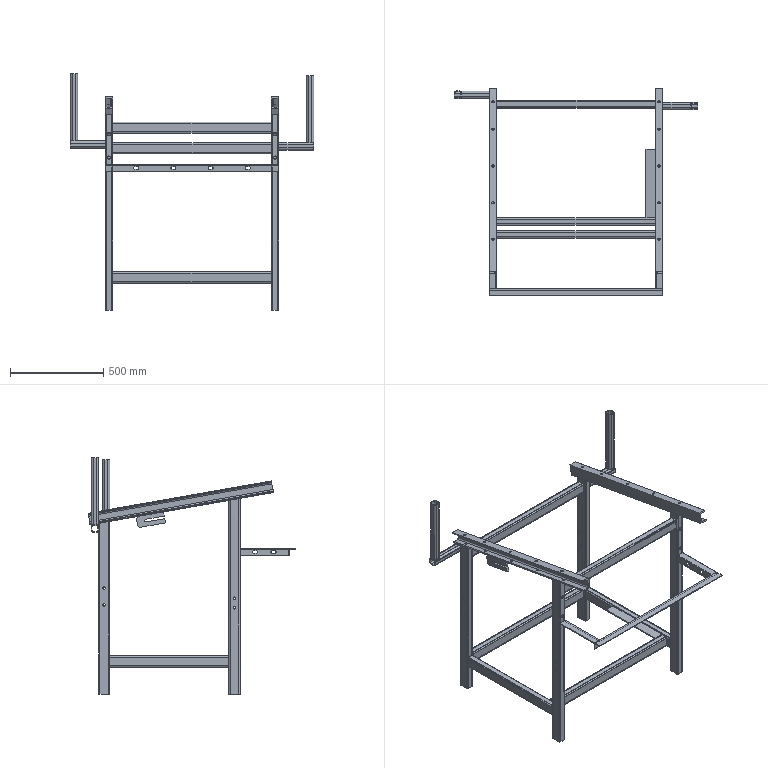Part | SolidWorks | features LayoutProfileFeature 1 | 21 solids | 455 faces | box 1308 x 1116 x 1270 mm | volume 7450780 mm3 | cylinder 238 | plane 217 | commonest cylinder face diameters 13 x76 15 x60 9 x40 16 x16 17 x16 24 x16